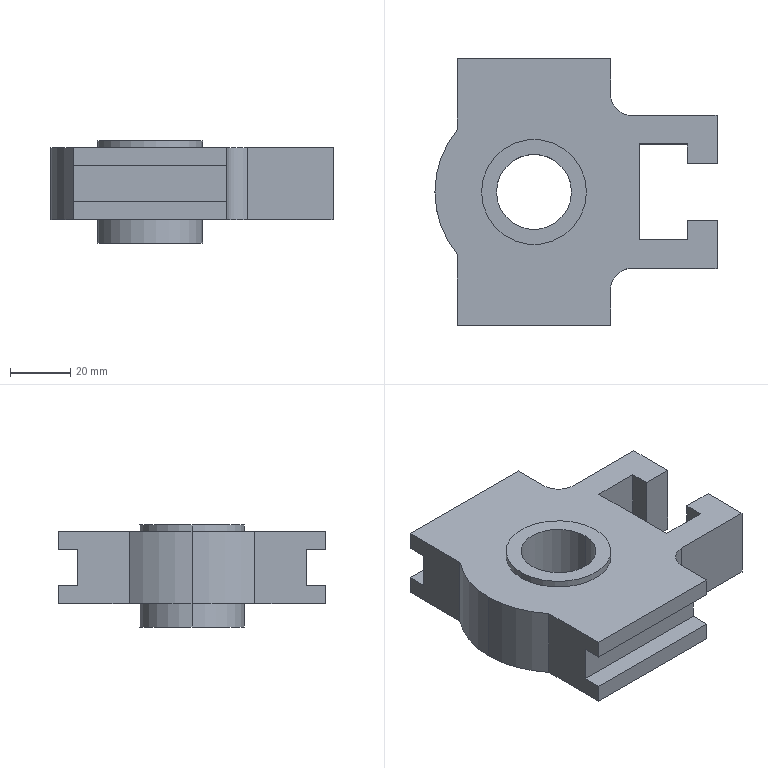Part | STEP file | UCT205 | 1 solid | 39 faces | box 94 x 89 x 34 mm | volume 126176 mm3 | plane 29 | cylinder 10 | commonest cylinder face diameters 35 x4 14.03 x2 25 x2 66 x2